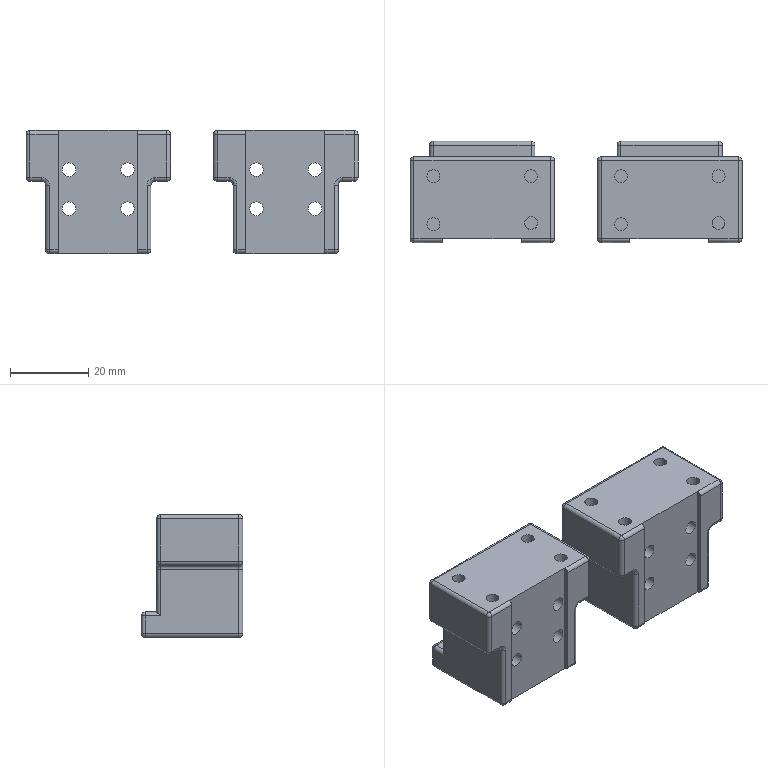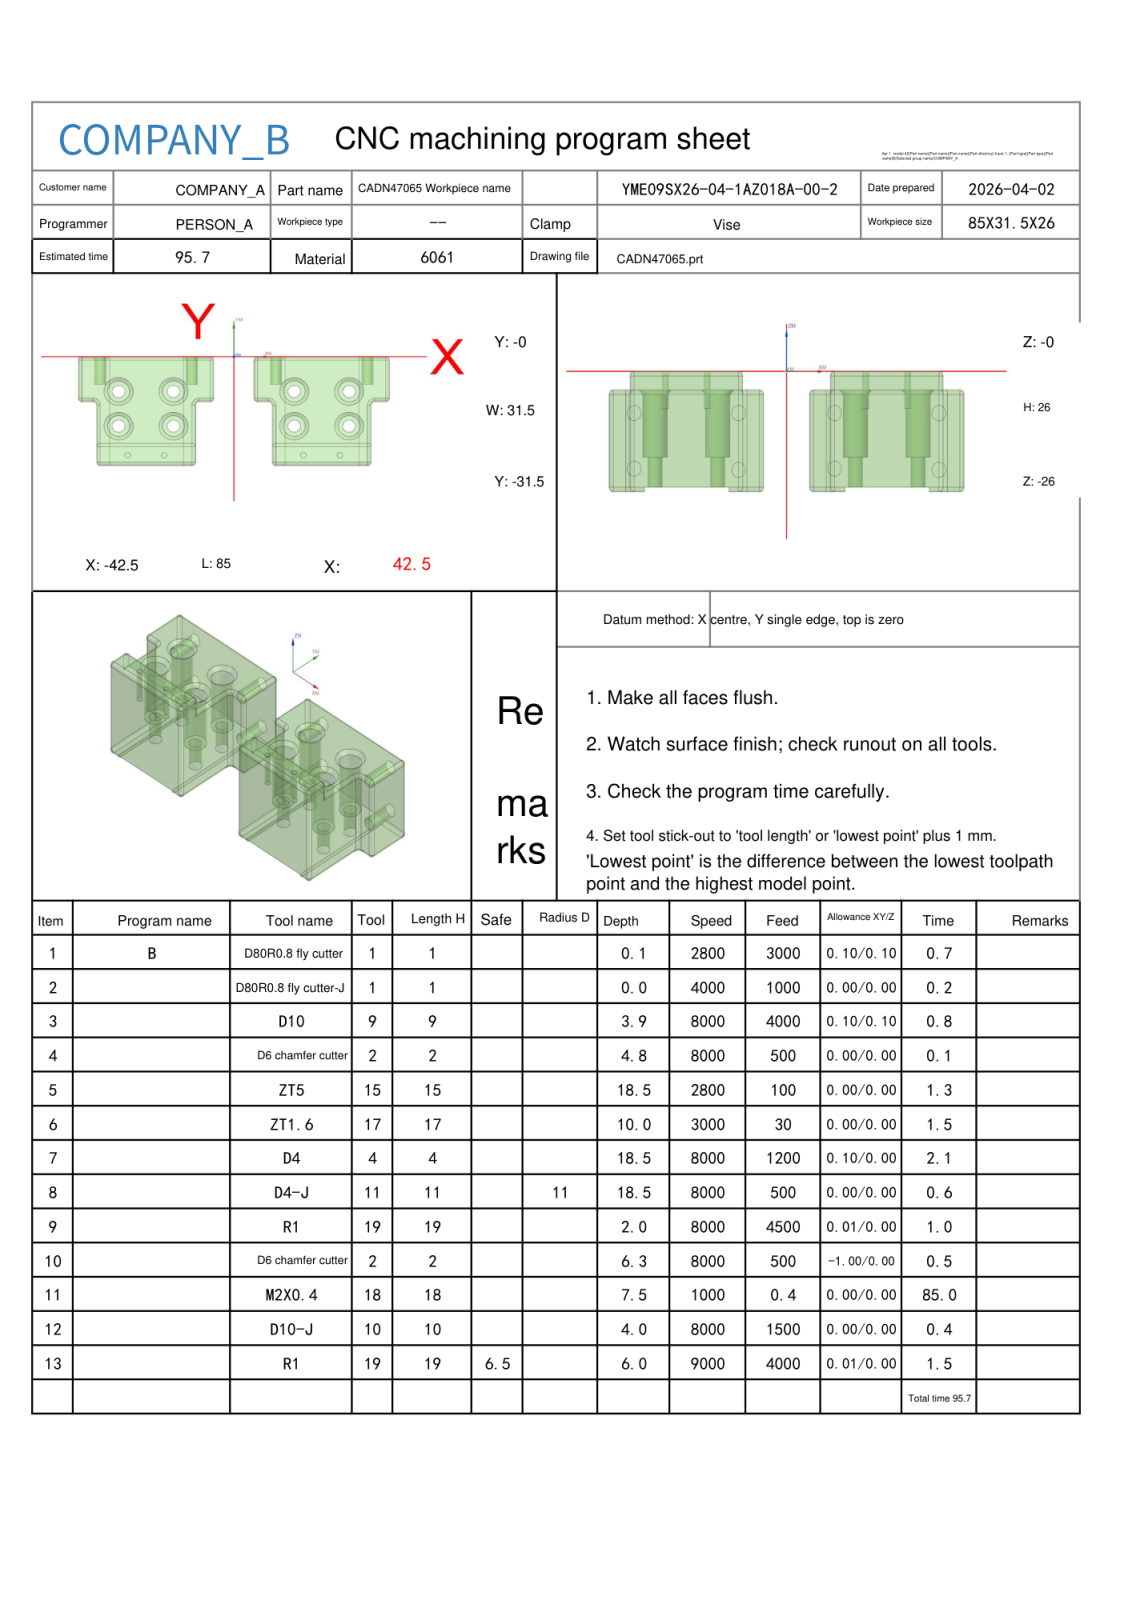NC program | NX | posted by the shop | part box 85 x 26 x 31.5 mm
Lines 1 to 1233 of 12542:
%
O0001
(Machine time: 173.10 MIN)
(===Total Tool:10===)
(T1=D80R0.8 fly cutter D=80.  R=0.8  D-  H01 Z=-0.   )
(T9=D10     D=10.  R=0.   D-  H09 Z=-3.9  )
(T2=D6 chamfer cutter   D=6.   R=0.   D-  H02 Z=-6.3  )
(T15=ZT5    D=5.   DR_a=118 D-  H15 Z=-18.51)
(T17=ZT1.6  D=1.6  DR_a=118 D-  H17 Z=-10.  )
(T4=D4      D=4.   R=0.   D-  H04 Z=-18.51)
(T11=D4-J   D=4.   R=0.   D11 H11 Z=-18.51)
(T19=R1     D=2.   R=1.   D-  H19 Z=-6.   )
(T18=M2X0.4 D=1.6  DR_a=180 D-  H18 Z=-7.5  )
(T10=D10-J  D=10.  R=0.   D10 H10 Z=-4.   )
G80 G90 G17 G49 G40
G91 G28 Z0
M01
N1 T01 M06
(D80R0.8 fly cutter  D=80. R=0.8 H=01 ce=0.10 di=0.10)
G00 G90 G54 X94.57 Y-13.688 M03 S2800
G43 H01 Z20.
M08
Z5.337
G01 Z3.337 F3000.
X82.551 Y-13.943
X-82.235 Y-17.444
X-94.29 Y-17.7
Z5.337
G00 X94.57 Y-13.688
Z4.875
G01 Z2.875
X82.551 Y-13.943
X-82.235 Y-17.444
X-94.29 Y-17.7
Z4.875
G00 X94.57 Y-13.688
Z4.412
G01 Z2.412
X82.551 Y-13.943
X-82.235 Y-17.444
X-94.29 Y-17.7
Z4.412
G00 X94.57 Y-13.688
Z3.95
G01 Z1.95
X82.551 Y-13.943
X-82.235 Y-17.444
X-94.29 Y-17.7
Z3.95
G00 Z20.
X94.57 Y-13.688
Z3.487
G01 Z1.487
X82.551 Y-13.943
X-82.235 Y-17.444
X-94.29 Y-17.7
Z3.487
G00 Z20.
X94.57 Y-13.688
Z3.025
G01 Z1.025
X82.551 Y-13.943
X-82.235 Y-17.444
X-94.29 Y-17.7
Z3.025
G00 Z20.
X94.57 Y-13.688
Z2.562
G01 Z.562
X82.551 Y-13.943
X-82.235 Y-17.444
X-94.29 Y-17.7
Z2.562
G00 Z20.
X94.57 Y-13.688
Z2.1
G01 Z.1
X82.551 Y-13.943
X-82.235 Y-17.444
X-94.29 Y-17.7
Z2.1
G00 Z20.
G91 G28 Z0.0
M05
M09
G91 G28 Z0.0
M01
N2 T01 M06
(D80R0.8 fly cutter-J  D=80. R=0.8 H=01 ce=0.00 di=0.00)
G00 G90 G54 X94.472 Y-13.691 M03 S4000
G43 H01 Z20.
M08
Z2.
G01 Z0.0 F1000.
X82.453 Y-13.947
X-82.136 Y-17.441
X-94.192 Y-17.696
Z2.
G00 Z20.
G91 G28 Z0.0
M05
M09
G91 G28 Z0.0
M01
N3 T09 M06
(D10  D=10. R=0. H=09 ce=0.10 di=0.10)
G00 G90 G54 X0.0 Y7. M03 S8000
G43 H09 Z13.8
M08
Z.943
G01 Z-.557 F4000.
Y3.9
X46.4
Y-16.9
X41.4
Y-20.659
Y-22.322
G03 X36.5 Y-19.855 I-4.9 J-3.633
G01 X11.5
G03 X6.6 Y-22.322 I0.0 J-6.1
G01 Y-16.9
X-6.6
Y-20.658
Y-22.322
G03 X-11.5 Y-19.855 I-4.9 J-3.633
G01 X-36.5
G03 X-41.4 Y-22.322 I0.0 J-6.1
G01 Y-20.659
Y-16.9
X-46.4
Y3.9
X-3.035
G02 X-2.203 Y3.455 I-.001 J-1.
G01 X2.203 Y-3.155
G03 X3.035 Y-3.6 I.832 J.555
G01 X37.903
G02 X38.9 Y-4.597 I-.003 J-1.
G01 Y-9.157
G02 X38.314 Y-10.064 I-1. J.003
G03 X35.714 Y-12.009 I3.086 J-6.836
G02 X34.96 Y-12.355 I-.756 J.654
G01 X13.04
G02 X12.286 Y-12.009 I.003 J1.
G03 X6.6 Y-9.4 I-5.686 J-4.891
G01 X-6.6
G03 X-12.286 Y-12.009 I0.0 J-7.5
G02 X-13.04 Y-12.355 I-.756 J.654
G01 X-34.96
G02 X-35.714 Y-12.009 I.003 J1.
G03 X-38.314 Y-10.064 I-5.686 J-4.891
G02 X-38.9 Y-9.157 I.414 J.91
G01 Y-4.597
G02 X-37.903 Y-3.6 I1. J-.003
G01 X0.0
X.5
Y7.
Z.943
G00 X0.0
Z.386
G01 Z-1.114
Y3.9
X46.4
Y-16.9
X41.4
Y-20.659
Y-22.322
G03 X36.5 Y-19.855 I-4.9 J-3.633
G01 X11.5
G03 X6.6 Y-22.322 I0.0 J-6.1
G01 Y-16.9
X-6.6
Y-20.658
Y-22.322
G03 X-11.5 Y-19.855 I-4.9 J-3.633
G01 X-36.5
G03 X-41.4 Y-22.322 I0.0 J-6.1
G01 Y-20.659
Y-16.9
X-46.4
Y3.9
X-3.035
G02 X-2.203 Y3.455 I-.001 J-1.
G01 X2.203 Y-3.155
G03 X3.035 Y-3.6 I.832 J.555
G01 X37.903
G02 X38.9 Y-4.597 I-.003 J-1.
G01 Y-9.157
G02 X38.314 Y-10.064 I-1. J.003
G03 X35.714 Y-12.009 I3.086 J-6.836
G02 X34.96 Y-12.355 I-.756 J.654
G01 X13.04
G02 X12.286 Y-12.009 I.003 J1.
G03 X6.6 Y-9.4 I-5.686 J-4.891
G01 X-6.6
G03 X-12.286 Y-12.009 I0.0 J-7.5
G02 X-13.04 Y-12.355 I-.756 J.654
G01 X-34.96
G02 X-35.714 Y-12.009 I.003 J1.
G03 X-38.314 Y-10.064 I-5.686 J-4.891
G02 X-38.9 Y-9.157 I.414 J.91
G01 Y-4.597
G02 X-37.903 Y-3.6 I1. J-.003
G01 X0.0
X.5
Y7.
Z.386
G00 X0.0
Z-.171
G01 Z-1.671
Y3.9
X46.4
Y-16.9
X41.4
Y-20.659
Y-22.322
G03 X36.5 Y-19.855 I-4.9 J-3.633
G01 X11.5
G03 X6.6 Y-22.322 I0.0 J-6.1
G01 Y-16.9
X-6.6
Y-20.658
Y-22.322
G03 X-11.5 Y-19.855 I-4.9 J-3.633
G01 X-36.5
G03 X-41.4 Y-22.322 I0.0 J-6.1
G01 Y-20.659
Y-16.9
X-46.4
Y3.9
X-3.035
G02 X-2.203 Y3.455 I-.001 J-1.
G01 X2.203 Y-3.155
G03 X3.035 Y-3.6 I.832 J.555
G01 X37.903
G02 X38.9 Y-4.597 I-.003 J-1.
G01 Y-9.157
G02 X38.314 Y-10.064 I-1. J.003
G03 X35.714 Y-12.009 I3.086 J-6.836
G02 X34.96 Y-12.355 I-.756 J.654
G01 X13.04
G02 X12.286 Y-12.009 I.003 J1.
G03 X6.6 Y-9.4 I-5.686 J-4.891
G01 X-6.6
G03 X-12.286 Y-12.009 I0.0 J-7.5
G02 X-13.04 Y-12.355 I-.756 J.654
G01 X-34.96
G02 X-35.714 Y-12.009 I.003 J1.
G03 X-38.314 Y-10.064 I-5.686 J-4.891
G02 X-38.9 Y-9.157 I.414 J.91
G01 Y-4.597
G02 X-37.903 Y-3.6 I1. J-.003
G01 X0.0
X.5
Y7.
Z-.171
G00 X0.0
Z-.729
G01 Z-2.229
Y3.9
X46.4
Y-16.9
X41.4
Y-20.659
Y-22.322
G03 X36.5 Y-19.855 I-4.9 J-3.633
G01 X11.5
G03 X6.6 Y-22.322 I0.0 J-6.1
G01 Y-16.9
X-6.6
Y-20.658
Y-22.322
G03 X-11.5 Y-19.855 I-4.9 J-3.633
G01 X-36.5
G03 X-41.4 Y-22.322 I0.0 J-6.1
G01 Y-20.659
Y-16.9
X-46.4
Y3.9
X-3.035
G02 X-2.203 Y3.455 I-.001 J-1.
G01 X2.203 Y-3.155
G03 X3.035 Y-3.6 I.832 J.555
G01 X37.903
G02 X38.9 Y-4.597 I-.003 J-1.
G01 Y-9.157
G02 X38.314 Y-10.064 I-1. J.003
G03 X35.714 Y-12.009 I3.086 J-6.836
G02 X34.96 Y-12.355 I-.756 J.654
G01 X13.04
G02 X12.286 Y-12.009 I.003 J1.
G03 X6.6 Y-9.4 I-5.686 J-4.891
G01 X-6.6
G03 X-12.286 Y-12.009 I0.0 J-7.5
G02 X-13.04 Y-12.355 I-.756 J.654
G01 X-34.96
G02 X-35.714 Y-12.009 I.003 J1.
G03 X-38.314 Y-10.064 I-5.686 J-4.891
G02 X-38.9 Y-9.157 I.414 J.91
G01 Y-4.597
G02 X-37.903 Y-3.6 I1. J-.003
G01 X0.0
X.5
Y7.
Z-.729
G00 X0.0
Z-1.286
G01 Z-2.786
Y3.9
X46.4
Y-16.9
X41.4
Y-20.659
Y-22.322
G03 X36.5 Y-19.855 I-4.9 J-3.633
G01 X11.5
G03 X6.6 Y-22.322 I0.0 J-6.1
G01 Y-16.9
X-6.6
Y-20.658
Y-22.322
G03 X-11.5 Y-19.855 I-4.9 J-3.633
G01 X-36.5
G03 X-41.4 Y-22.322 I0.0 J-6.1
G01 Y-20.659
Y-16.9
X-46.4
Y3.9
X-3.035
G02 X-2.203 Y3.455 I-.001 J-1.
G01 X2.203 Y-3.155
G03 X3.035 Y-3.6 I.832 J.555
G01 X37.903
G02 X38.9 Y-4.597 I-.003 J-1.
G01 Y-9.157
G02 X38.314 Y-10.064 I-1. J.003
G03 X35.714 Y-12.009 I3.086 J-6.836
G02 X34.96 Y-12.355 I-.756 J.654
G01 X13.04
G02 X12.286 Y-12.009 I.003 J1.
G03 X6.6 Y-9.4 I-5.686 J-4.891
G01 X-6.6
G03 X-12.286 Y-12.009 I0.0 J-7.5
G02 X-13.04 Y-12.355 I-.756 J.654
G01 X-34.96
G02 X-35.714 Y-12.009 I.003 J1.
G03 X-38.314 Y-10.064 I-5.686 J-4.891
G02 X-38.9 Y-9.157 I.414 J.91
G01 Y-4.597
G02 X-37.903 Y-3.6 I1. J-.003
G01 X0.0
X.5
Y7.
Z-1.286
G00 X0.0
Z-1.843
G01 Z-3.343
Y3.9
X46.4
Y-16.9
X41.4
Y-20.659
Y-22.322
G03 X36.5 Y-19.855 I-4.9 J-3.633
G01 X11.5
G03 X6.6 Y-22.322 I0.0 J-6.1
G01 Y-16.9
X-6.6
Y-20.658
Y-22.322
G03 X-11.5 Y-19.855 I-4.9 J-3.633
G01 X-36.5
G03 X-41.4 Y-22.322 I0.0 J-6.1
G01 Y-20.659
Y-16.9
X-46.4
Y3.9
X-3.035
G02 X-2.203 Y3.455 I-.001 J-1.
G01 X2.203 Y-3.155
G03 X3.035 Y-3.6 I.832 J.555
G01 X37.903
G02 X38.9 Y-4.597 I-.003 J-1.
G01 Y-9.157
G02 X38.314 Y-10.064 I-1. J.003
G03 X35.714 Y-12.009 I3.086 J-6.836
G02 X34.96 Y-12.355 I-.756 J.654
G01 X13.04
G02 X12.286 Y-12.009 I.003 J1.
G03 X6.6 Y-9.4 I-5.686 J-4.891
G01 X-6.6
G03 X-12.286 Y-12.009 I0.0 J-7.5
G02 X-13.04 Y-12.355 I-.756 J.654
G01 X-34.96
G02 X-35.714 Y-12.009 I.003 J1.
G03 X-38.314 Y-10.064 I-5.686 J-4.891
G02 X-38.9 Y-9.157 I.414 J.91
G01 Y-4.597
G02 X-37.903 Y-3.6 I1. J-.003
G01 X0.0
X.5
Y7.
Z-1.843
G00 X0.0
Z-2.4
G01 Z-3.9
Y3.9
X46.4
Y-16.9
X41.4
Y-20.659
Y-22.322
G03 X36.5 Y-19.855 I-4.9 J-3.633
G01 X11.5
G03 X6.6 Y-22.322 I0.0 J-6.1
G01 Y-16.9
X-6.6
Y-20.658
Y-22.322
G03 X-11.5 Y-19.855 I-4.9 J-3.633
G01 X-36.5
G03 X-41.4 Y-22.322 I0.0 J-6.1
G01 Y-20.659
Y-16.9
X-46.4
Y3.9
X-3.035
G02 X-2.203 Y3.455 I-.001 J-1.
G01 X2.203 Y-3.155
G03 X3.035 Y-3.6 I.832 J.555
G01 X37.903
G02 X38.9 Y-4.597 I-.003 J-1.
G01 Y-9.157
G02 X38.314 Y-10.064 I-1. J.003
G03 X35.714 Y-12.009 I3.086 J-6.836
G02 X34.96 Y-12.355 I-.756 J.654
G01 X13.04
G02 X12.286 Y-12.009 I.003 J1.
G03 X6.6 Y-9.4 I-5.686 J-4.891
G01 X-6.6
G03 X-12.286 Y-12.009 I0.0 J-7.5
G02 X-13.04 Y-12.355 I-.756 J.654
G01 X-34.96
G02 X-35.714 Y-12.009 I.003 J1.
G03 X-38.314 Y-10.064 I-5.686 J-4.891
G02 X-38.9 Y-9.157 I.414 J.91
G01 Y-4.597
G02 X-37.903 Y-3.6 I1. J-.003
G01 X0.0
X.5
Y7.
Z-2.4
G00 Z13.8
G91 G28 Z0.0
M05
M09
G91 G28 Z0.0
M01
N4 T02 M06
(D6 chamfer cutter  D=6. R=0. H=02 ce=0.00 di=0.10)
G00 G90 G54 X-31.502 Y-10.05 M03 S8000
G43 H02 Z20.
M08
G98 G81 X-31.502 Y-10.05 Z-4.8 R-3. F500.
Y-20.05
X-29.011 Y-28.455 Z-.8 R1.
X-19.011
X-16.502 Y-20.05 Z-4.8 R-3.
Y-10.05
X16.498
Y-20.05
X18.989 Y-28.455 Z-.8 R1.
X28.989
X31.498 Y-20.05 Z-4.8 R-3.
Y-10.05
G80
G00 Z20.
G91 G28 Z0.0
M05
M09
G91 G28 Z0.0
M01
N5 T15 M06
(ZT5 D=5. DR_a=118 H=15)
G00 G90 G54 X-31.502 Y-20.05 M03 S2800
G43 H15 Z20.
M08
G98 G83 X-31.502 Y-20.05 Z-18.51 R-3. F100. Q2.
Y-10.05
X-16.502
Y-20.05
X16.498
Y-10.05
X31.498
Y-20.05
G80
G00 Z20.
G91 G28 Z0.0
M05
M09
G91 G28 Z0.0
M01
N6 T17 M06
(ZT1.6 D=1.6 DR_a=118 H=17)
G00 G90 G54 X-29.011 Y-28.455 M03 S3000
G43 H17 Z20.
M08
G98 G83 X-29.011 Y-28.455 Z-10. R1. F30. Q1.
X-19.011
X18.989
X28.989
G80
G00 Z20.
G91 G28 Z0.0
M05
M09
G91 G28 Z0.0
M01
N7 T04 M06
(D4  D=4. R=0. H=04 ce=0.10 di=0.00)
G00 G90 G54 X-16.502 Y-10.05 M03 S8000
G43 H04 Z20.
M08
Z-2.5
G03 X-16.952 Y-9.6 I-.45 J0.0 F1200.
X-17.402 Y-10.05 I0.0 J-.45
X-17.402 Y-10.05 Z-2.8 I.9 J0.0
X-17.402 Y-10.05 Z-3.1 I.9 J0.0
X-17.402 Y-10.05 Z-3.4 I.9 J0.0
X-17.402 Y-10.05 Z-3.7 I.9 J0.0
X-17.402 Y-10.05 Z-4. I.9 J0.0
X-17.402 Y-10.05 Z-4.3 I.9 J0.0
X-17.402 Y-10.05 Z-4.6 I.9 J0.0
X-17.402 Y-10.05 Z-4.9 I.9 J0.0
X-17.402 Y-10.05 Z-5.2 I.9 J0.0
X-17.402 Y-10.05 Z-5.5 I.9 J0.0
X-17.402 Y-10.05 Z-5.8 I.9 J0.0
X-17.402 Y-10.05 Z-6.1 I.9 J0.0
X-17.402 Y-10.05 Z-6.4 I.9 J0.0
X-17.402 Y-10.05 Z-6.7 I.9 J0.0
X-17.402 Y-10.05 Z-7. I.9 J0.0
X-17.402 Y-10.05 Z-7.3 I.9 J0.0
X-17.402 Y-10.05 Z-7.6 I.9 J0.0
X-17.402 Y-10.05 Z-7.9 I.9 J0.0
X-17.402 Y-10.05 Z-8.2 I.9 J0.0
X-17.402 Y-10.05 Z-8.5 I.9 J0.0
X-17.402 Y-10.05 Z-8.8 I.9 J0.0
X-17.402 Y-10.05 Z-9.1 I.9 J0.0
X-17.402 Y-10.05 Z-9.4 I.9 J0.0
X-17.402 Y-10.05 Z-9.7 I.9 J0.0
X-17.402 Y-10.05 Z-10. I.9 J0.0
X-17.402 Y-10.05 Z-10.3 I.9 J0.0
X-17.402 Y-10.05 Z-10.6 I.9 J0.0
X-17.402 Y-10.05 Z-10.9 I.9 J0.0
X-17.402 Y-10.05 Z-11.2 I.9 J0.0
X-17.402 Y-10.05 Z-11.5 I.9 J0.0
X-17.402 Y-10.05 Z-11.8 I.9 J0.0
X-17.402 Y-10.05 Z-12.1 I.9 J0.0
X-17.402 Y-10.05 Z-12.4 I.9 J0.0
X-17.402 Y-10.05 Z-12.7 I.9 J0.0
X-17.402 Y-10.05 Z-13. I.9 J0.0
X-17.402 Y-10.05 Z-13.3 I.9 J0.0
X-17.402 Y-10.05 Z-13.6 I.9 J0.0
X-17.402 Y-10.05 Z-13.9 I.9 J0.0
X-17.402 Y-10.05 Z-14.2 I.9 J0.0
X-17.402 Y-10.05 Z-14.5 I.9 J0.0
X-17.402 Y-10.05 Z-14.8 I.9 J0.0
X-17.402 Y-10.05 Z-15.1 I.9 J0.0
X-17.402 Y-10.05 Z-15.4 I.9 J0.0
X-17.402 Y-10.05 Z-15.7 I.9 J0.0
X-17.402 Y-10.05 Z-16. I.9 J0.0
X-17.402 Y-10.05 Z-16.3 I.9 J0.0
X-17.402 Y-10.05 Z-16.6 I.9 J0.0
X-17.402 Y-10.05 Z-16.9 I.9 J0.0
X-17.402 Y-10.05 Z-17.2 I.9 J0.0
X-17.402 Y-10.05 Z-17.5 I.9 J0.0
X-17.402 Y-10.05 Z-17.8 I.9 J0.0
X-17.402 Y-10.05 Z-18.1 I.9 J0.0
X-17.402 Y-10.05 Z-18.4 I.9 J0.0
X-15.901 Y-10.719 Z-18.51 I.9 J0.0
X-15.602 Y-10.05 I-.602 J.669
X-16.502 Y-9.15 I-.9 J0.0
X-17.402 Y-10.05 I0.0 J-.9
X-16.502 Y-10.95 I.9 J0.0
X-15.901 Y-10.719 I0.0 J.9
X-15.752 Y-10.385 I-.301 J.335
X-16.202 Y-9.935 I-.45 J0.0
X-16.502 Y-10.05 I0.0 J-.45
G00 Z20.
X-31.502
Z-2.5
G03 X-31.952 Y-9.6 I-.45 J0.0
X-32.402 Y-10.05 I0.0 J-.45
X-32.402 Y-10.05 Z-2.8 I.9 J0.0
X-32.402 Y-10.05 Z-3.1 I.9 J0.0
X-32.402 Y-10.05 Z-3.4 I.9 J0.0
X-32.402 Y-10.05 Z-3.7 I.9 J0.0
X-32.402 Y-10.05 Z-4. I.9 J0.0
X-32.402 Y-10.05 Z-4.3 I.9 J0.0
X-32.402 Y-10.05 Z-4.6 I.9 J0.0
X-32.402 Y-10.05 Z-4.9 I.9 J0.0
X-32.402 Y-10.05 Z-5.2 I.9 J0.0
X-32.402 Y-10.05 Z-5.5 I.9 J0.0
X-32.402 Y-10.05 Z-5.8 I.9 J0.0
X-32.402 Y-10.05 Z-6.1 I.9 J0.0
X-32.402 Y-10.05 Z-6.4 I.9 J0.0
X-32.402 Y-10.05 Z-6.7 I.9 J0.0
X-32.402 Y-10.05 Z-7. I.9 J0.0
X-32.402 Y-10.05 Z-7.3 I.9 J0.0
X-32.402 Y-10.05 Z-7.6 I.9 J0.0
X-32.402 Y-10.05 Z-7.9 I.9 J0.0
X-32.402 Y-10.05 Z-8.2 I.9 J0.0
X-32.402 Y-10.05 Z-8.5 I.9 J0.0
X-32.402 Y-10.05 Z-8.8 I.9 J0.0
X-32.402 Y-10.05 Z-9.1 I.9 J0.0
X-32.402 Y-10.05 Z-9.4 I.9 J0.0
X-32.402 Y-10.05 Z-9.7 I.9 J0.0
X-32.402 Y-10.05 Z-10. I.9 J0.0
X-32.402 Y-10.05 Z-10.3 I.9 J0.0
X-32.402 Y-10.05 Z-10.6 I.9 J0.0
X-32.402 Y-10.05 Z-10.9 I.9 J0.0
X-32.402 Y-10.05 Z-11.2 I.9 J0.0
X-32.402 Y-10.05 Z-11.5 I.9 J0.0
X-32.402 Y-10.05 Z-11.8 I.9 J0.0
X-32.402 Y-10.05 Z-12.1 I.9 J0.0
X-32.402 Y-10.05 Z-12.4 I.9 J0.0
X-32.402 Y-10.05 Z-12.7 I.9 J0.0
X-32.402 Y-10.05 Z-13. I.9 J0.0
X-32.402 Y-10.05 Z-13.3 I.9 J0.0
X-32.402 Y-10.05 Z-13.6 I.9 J0.0
X-32.402 Y-10.05 Z-13.9 I.9 J0.0
X-32.402 Y-10.05 Z-14.2 I.9 J0.0
X-32.402 Y-10.05 Z-14.5 I.9 J0.0
X-32.402 Y-10.05 Z-14.8 I.9 J0.0
X-32.402 Y-10.05 Z-15.1 I.9 J0.0
X-32.402 Y-10.05 Z-15.4 I.9 J0.0
X-32.402 Y-10.05 Z-15.7 I.9 J0.0
X-32.402 Y-10.05 Z-16. I.9 J0.0
X-32.402 Y-10.05 Z-16.3 I.9 J0.0
X-32.402 Y-10.05 Z-16.6 I.9 J0.0
X-32.402 Y-10.05 Z-16.9 I.9 J0.0
X-32.402 Y-10.05 Z-17.2 I.9 J0.0
X-32.402 Y-10.05 Z-17.5 I.9 J0.0
X-32.402 Y-10.05 Z-17.8 I.9 J0.0
X-32.402 Y-10.05 Z-18.1 I.9 J0.0
X-32.402 Y-10.05 Z-18.4 I.9 J0.0
X-30.901 Y-10.719 Z-18.51 I.9 J0.0
X-30.602 Y-10.05 I-.602 J.669
X-31.502 Y-9.15 I-.9 J0.0
X-32.402 Y-10.05 I0.0 J-.9
X-31.502 Y-10.95 I.9 J0.0
X-30.901 Y-10.719 I0.0 J.9
X-30.752 Y-10.385 I-.301 J.335
X-31.202 Y-9.935 I-.45 J0.0
X-31.502 Y-10.05 I0.0 J-.45
G00 Z20.
Y-20.05
Z-2.5
G03 X-31.952 Y-19.6 I-.45 J0.0
X-32.402 Y-20.05 I0.0 J-.45
X-32.402 Y-20.05 Z-2.8 I.9 J0.0
X-32.402 Y-20.05 Z-3.1 I.9 J0.0
X-32.402 Y-20.05 Z-3.4 I.9 J0.0
X-32.402 Y-20.05 Z-3.7 I.9 J0.0
X-32.402 Y-20.05 Z-4. I.9 J0.0
X-32.402 Y-20.05 Z-4.3 I.9 J0.0
X-32.402 Y-20.05 Z-4.6 I.9 J0.0
X-32.402 Y-20.05 Z-4.9 I.9 J0.0
X-32.402 Y-20.05 Z-5.2 I.9 J0.0
X-32.402 Y-20.05 Z-5.5 I.9 J0.0
X-32.402 Y-20.05 Z-5.8 I.9 J0.0
X-32.402 Y-20.05 Z-6.1 I.9 J0.0
X-32.402 Y-20.05 Z-6.4 I.9 J0.0
X-32.402 Y-20.05 Z-6.7 I.9 J0.0
X-32.402 Y-20.05 Z-7. I.9 J0.0
X-32.402 Y-20.05 Z-7.3 I.9 J0.0
X-32.402 Y-20.05 Z-7.6 I.9 J0.0
X-32.402 Y-20.05 Z-7.9 I.9 J0.0
X-32.402 Y-20.05 Z-8.2 I.9 J0.0
X-32.402 Y-20.05 Z-8.5 I.9 J0.0
X-32.402 Y-20.05 Z-8.8 I.9 J0.0
X-32.402 Y-20.05 Z-9.1 I.9 J0.0
X-32.402 Y-20.05 Z-9.4 I.9 J0.0
X-32.402 Y-20.05 Z-9.7 I.9 J0.0
X-32.402 Y-20.05 Z-10. I.9 J0.0
X-32.402 Y-20.05 Z-10.3 I.9 J0.0
X-32.402 Y-20.05 Z-10.6 I.9 J0.0
X-32.402 Y-20.05 Z-10.9 I.9 J0.0
X-32.402 Y-20.05 Z-11.2 I.9 J0.0
X-32.402 Y-20.05 Z-11.5 I.9 J0.0
X-32.402 Y-20.05 Z-11.8 I.9 J0.0
X-32.402 Y-20.05 Z-12.1 I.9 J0.0
X-32.402 Y-20.05 Z-12.4 I.9 J0.0
X-32.402 Y-20.05 Z-12.7 I.9 J0.0
X-32.402 Y-20.05 Z-13. I.9 J0.0
X-32.402 Y-20.05 Z-13.3 I.9 J0.0
X-32.402 Y-20.05 Z-13.6 I.9 J0.0
X-32.402 Y-20.05 Z-13.9 I.9 J0.0
X-32.402 Y-20.05 Z-14.2 I.9 J0.0
X-32.402 Y-20.05 Z-14.5 I.9 J0.0
X-32.402 Y-20.05 Z-14.8 I.9 J0.0
X-32.402 Y-20.05 Z-15.1 I.9 J0.0
X-32.402 Y-20.05 Z-15.4 I.9 J0.0
X-32.402 Y-20.05 Z-15.7 I.9 J0.0
X-32.402 Y-20.05 Z-16. I.9 J0.0
X-32.402 Y-20.05 Z-16.3 I.9 J0.0
X-32.402 Y-20.05 Z-16.6 I.9 J0.0
X-32.402 Y-20.05 Z-16.9 I.9 J0.0
X-32.402 Y-20.05 Z-17.2 I.9 J0.0
X-32.402 Y-20.05 Z-17.5 I.9 J0.0
X-32.402 Y-20.05 Z-17.8 I.9 J0.0
X-32.402 Y-20.05 Z-18.1 I.9 J0.0
X-32.402 Y-20.05 Z-18.4 I.9 J0.0
X-30.901 Y-20.719 Z-18.51 I.9 J0.0
X-30.602 Y-20.05 I-.602 J.669
X-31.502 Y-19.15 I-.9 J0.0
X-32.402 Y-20.05 I0.0 J-.9
X-31.502 Y-20.95 I.9 J0.0
X-30.901 Y-20.719 I0.0 J.9
X-30.752 Y-20.385 I-.301 J.335
X-31.202 Y-19.935 I-.45 J0.0
X-31.502 Y-20.05 I0.0 J-.45
G00 Z20.
X-16.502
Z-2.5
G03 X-16.952 Y-19.6 I-.45 J0.0
X-17.402 Y-20.05 I0.0 J-.45
X-17.402 Y-20.05 Z-2.8 I.9 J0.0
X-17.402 Y-20.05 Z-3.1 I.9 J0.0
X-17.402 Y-20.05 Z-3.4 I.9 J0.0
X-17.402 Y-20.05 Z-3.7 I.9 J0.0
X-17.402 Y-20.05 Z-4. I.9 J0.0
X-17.402 Y-20.05 Z-4.3 I.9 J0.0
X-17.402 Y-20.05 Z-4.6 I.9 J0.0
X-17.402 Y-20.05 Z-4.9 I.9 J0.0
X-17.402 Y-20.05 Z-5.2 I.9 J0.0
X-17.402 Y-20.05 Z-5.5 I.9 J0.0
X-17.402 Y-20.05 Z-5.8 I.9 J0.0
X-17.402 Y-20.05 Z-6.1 I.9 J0.0
X-17.402 Y-20.05 Z-6.4 I.9 J0.0
X-17.402 Y-20.05 Z-6.7 I.9 J0.0
X-17.402 Y-20.05 Z-7. I.9 J0.0
X-17.402 Y-20.05 Z-7.3 I.9 J0.0
X-17.402 Y-20.05 Z-7.6 I.9 J0.0
X-17.402 Y-20.05 Z-7.9 I.9 J0.0
X-17.402 Y-20.05 Z-8.2 I.9 J0.0
X-17.402 Y-20.05 Z-8.5 I.9 J0.0
X-17.402 Y-20.05 Z-8.8 I.9 J0.0
X-17.402 Y-20.05 Z-9.1 I.9 J0.0
X-17.402 Y-20.05 Z-9.4 I.9 J0.0
X-17.402 Y-20.05 Z-9.7 I.9 J0.0
X-17.402 Y-20.05 Z-10. I.9 J0.0
X-17.402 Y-20.05 Z-10.3 I.9 J0.0
X-17.402 Y-20.05 Z-10.6 I.9 J0.0
X-17.402 Y-20.05 Z-10.9 I.9 J0.0
X-17.402 Y-20.05 Z-11.2 I.9 J0.0
X-17.402 Y-20.05 Z-11.5 I.9 J0.0
X-17.402 Y-20.05 Z-11.8 I.9 J0.0
X-17.402 Y-20.05 Z-12.1 I.9 J0.0
X-17.402 Y-20.05 Z-12.4 I.9 J0.0
X-17.402 Y-20.05 Z-12.7 I.9 J0.0
X-17.402 Y-20.05 Z-13. I.9 J0.0
X-17.402 Y-20.05 Z-13.3 I.9 J0.0
X-17.402 Y-20.05 Z-13.6 I.9 J0.0
X-17.402 Y-20.05 Z-13.9 I.9 J0.0
X-17.402 Y-20.05 Z-14.2 I.9 J0.0
X-17.402 Y-20.05 Z-14.5 I.9 J0.0
X-17.402 Y-20.05 Z-14.8 I.9 J0.0
X-17.402 Y-20.05 Z-15.1 I.9 J0.0
X-17.402 Y-20.05 Z-15.4 I.9 J0.0
X-17.402 Y-20.05 Z-15.7 I.9 J0.0
X-17.402 Y-20.05 Z-16. I.9 J0.0
X-17.402 Y-20.05 Z-16.3 I.9 J0.0
X-17.402 Y-20.05 Z-16.6 I.9 J0.0
X-17.402 Y-20.05 Z-16.9 I.9 J0.0
X-17.402 Y-20.05 Z-17.2 I.9 J0.0
X-17.402 Y-20.05 Z-17.5 I.9 J0.0
X-17.402 Y-20.05 Z-17.8 I.9 J0.0
X-17.402 Y-20.05 Z-18.1 I.9 J0.0
X-17.402 Y-20.05 Z-18.4 I.9 J0.0
X-15.901 Y-20.719 Z-18.51 I.9 J0.0
X-15.602 Y-20.05 I-.602 J.669
X-16.502 Y-19.15 I-.9 J0.0
X-17.402 Y-20.05 I0.0 J-.9
X-16.502 Y-20.95 I.9 J0.0
X-15.901 Y-20.719 I0.0 J.9
X-15.752 Y-20.385 I-.301 J.335
X-16.202 Y-19.935 I-.45 J0.0
X-16.502 Y-20.05 I0.0 J-.45
G00 Z20.
X16.498
Z-2.5
G03 X16.048 Y-19.6 I-.45 J0.0
X15.598 Y-20.05 I0.0 J-.45
X15.598 Y-20.05 Z-2.8 I.9 J0.0
X15.598 Y-20.05 Z-3.1 I.9 J0.0
X15.598 Y-20.05 Z-3.4 I.9 J0.0
X15.598 Y-20.05 Z-3.7 I.9 J0.0
X15.598 Y-20.05 Z-4. I.9 J0.0
X15.598 Y-20.05 Z-4.3 I.9 J0.0
X15.598 Y-20.05 Z-4.6 I.9 J0.0
X15.598 Y-20.05 Z-4.9 I.9 J0.0
X15.598 Y-20.05 Z-5.2 I.9 J0.0
X15.598 Y-20.05 Z-5.5 I.9 J0.0
X15.598 Y-20.05 Z-5.8 I.9 J0.0
X15.598 Y-20.05 Z-6.1 I.9 J0.0
X15.598 Y-20.05 Z-6.4 I.9 J0.0
X15.598 Y-20.05 Z-6.7 I.9 J0.0
X15.598 Y-20.05 Z-7. I.9 J0.0
X15.598 Y-20.05 Z-7.3 I.9 J0.0
X15.598 Y-20.05 Z-7.6 I.9 J0.0
X15.598 Y-20.05 Z-7.9 I.9 J0.0
X15.598 Y-20.05 Z-8.2 I.9 J0.0
X15.598 Y-20.05 Z-8.5 I.9 J0.0
X15.598 Y-20.05 Z-8.8 I.9 J0.0
X15.598 Y-20.05 Z-9.1 I.9 J0.0
X15.598 Y-20.05 Z-9.4 I.9 J0.0
X15.598 Y-20.05 Z-9.7 I.9 J0.0
X15.598 Y-20.05 Z-10. I.9 J0.0
X15.598 Y-20.05 Z-10.3 I.9 J0.0
X15.598 Y-20.05 Z-10.6 I.9 J0.0
X15.598 Y-20.05 Z-10.9 I.9 J0.0
X15.598 Y-20.05 Z-11.2 I.9 J0.0
X15.598 Y-20.05 Z-11.5 I.9 J0.0
X15.598 Y-20.05 Z-11.8 I.9 J0.0
X15.598 Y-20.05 Z-12.1 I.9 J0.0
X15.598 Y-20.05 Z-12.4 I.9 J0.0
X15.598 Y-20.05 Z-12.7 I.9 J0.0
X15.598 Y-20.05 Z-13. I.9 J0.0
X15.598 Y-20.05 Z-13.3 I.9 J0.0
X15.598 Y-20.05 Z-13.6 I.9 J0.0
X15.598 Y-20.05 Z-13.9 I.9 J0.0
X15.598 Y-20.05 Z-14.2 I.9 J0.0
X15.598 Y-20.05 Z-14.5 I.9 J0.0
X15.598 Y-20.05 Z-14.8 I.9 J0.0
X15.598 Y-20.05 Z-15.1 I.9 J0.0
X15.598 Y-20.05 Z-15.4 I.9 J0.0
X15.598 Y-20.05 Z-15.7 I.9 J0.0
X15.598 Y-20.05 Z-16. I.9 J0.0
X15.598 Y-20.05 Z-16.3 I.9 J0.0
X15.598 Y-20.05 Z-16.6 I.9 J0.0
X15.598 Y-20.05 Z-16.9 I.9 J0.0
X15.598 Y-20.05 Z-17.2 I.9 J0.0
X15.598 Y-20.05 Z-17.5 I.9 J0.0
X15.598 Y-20.05 Z-17.8 I.9 J0.0
X15.598 Y-20.05 Z-18.1 I.9 J0.0
X15.598 Y-20.05 Z-18.4 I.9 J0.0
X17.099 Y-20.719 Z-18.51 I.9 J0.0
X17.398 Y-20.05 I-.602 J.669
X16.498 Y-19.15 I-.9 J0.0
X15.598 Y-20.05 I0.0 J-.9
X16.498 Y-20.95 I.9 J0.0
X17.099 Y-20.719 I0.0 J.9
X17.248 Y-20.385 I-.301 J.335
X16.798 Y-19.935 I-.45 J0.0
X16.498 Y-20.05 I0.0 J-.45
G00 Z20.
Y-10.05
Z-2.5
G03 X16.048 Y-9.6 I-.45 J0.0
X15.598 Y-10.05 I0.0 J-.45
X15.598 Y-10.05 Z-2.8 I.9 J0.0
X15.598 Y-10.05 Z-3.1 I.9 J0.0
X15.598 Y-10.05 Z-3.4 I.9 J0.0
X15.598 Y-10.05 Z-3.7 I.9 J0.0
X15.598 Y-10.05 Z-4. I.9 J0.0
X15.598 Y-10.05 Z-4.3 I.9 J0.0
X15.598 Y-10.05 Z-4.6 I.9 J0.0
X15.598 Y-10.05 Z-4.9 I.9 J0.0
X15.598 Y-10.05 Z-5.2 I.9 J0.0
X15.598 Y-10.05 Z-5.5 I.9 J0.0
X15.598 Y-10.05 Z-5.8 I.9 J0.0
X15.598 Y-10.05 Z-6.1 I.9 J0.0
X15.598 Y-10.05 Z-6.4 I.9 J0.0
X15.598 Y-10.05 Z-6.7 I.9 J0.0
X15.598 Y-10.05 Z-7. I.9 J0.0
X15.598 Y-10.05 Z-7.3 I.9 J0.0
X15.598 Y-10.05 Z-7.6 I.9 J0.0
X15.598 Y-10.05 Z-7.9 I.9 J0.0
X15.598 Y-10.05 Z-8.2 I.9 J0.0
X15.598 Y-10.05 Z-8.5 I.9 J0.0
X15.598 Y-10.05 Z-8.8 I.9 J0.0
X15.598 Y-10.05 Z-9.1 I.9 J0.0
X15.598 Y-10.05 Z-9.4 I.9 J0.0
X15.598 Y-10.05 Z-9.7 I.9 J0.0
X15.598 Y-10.05 Z-10. I.9 J0.0
X15.598 Y-10.05 Z-10.3 I.9 J0.0
X15.598 Y-10.05 Z-10.6 I.9 J0.0
X15.598 Y-10.05 Z-10.9 I.9 J0.0
X15.598 Y-10.05 Z-11.2 I.9 J0.0
X15.598 Y-10.05 Z-11.5 I.9 J0.0
X15.598 Y-10.05 Z-11.8 I.9 J0.0
X15.598 Y-10.05 Z-12.1 I.9 J0.0
X15.598 Y-10.05 Z-12.4 I.9 J0.0
X15.598 Y-10.05 Z-12.7 I.9 J0.0
X15.598 Y-10.05 Z-13. I.9 J0.0
X15.598 Y-10.05 Z-13.3 I.9 J0.0
X15.598 Y-10.05 Z-13.6 I.9 J0.0
X15.598 Y-10.05 Z-13.9 I.9 J0.0
X15.598 Y-10.05 Z-14.2 I.9 J0.0
X15.598 Y-10.05 Z-14.5 I.9 J0.0
X15.598 Y-10.05 Z-14.8 I.9 J0.0
X15.598 Y-10.05 Z-15.1 I.9 J0.0
X15.598 Y-10.05 Z-15.4 I.9 J0.0
X15.598 Y-10.05 Z-15.7 I.9 J0.0
X15.598 Y-10.05 Z-16. I.9 J0.0
X15.598 Y-10.05 Z-16.3 I.9 J0.0
X15.598 Y-10.05 Z-16.6 I.9 J0.0
X15.598 Y-10.05 Z-16.9 I.9 J0.0
X15.598 Y-10.05 Z-17.2 I.9 J0.0
X15.598 Y-10.05 Z-17.5 I.9 J0.0
X15.598 Y-10.05 Z-17.8 I.9 J0.0
X15.598 Y-10.05 Z-18.1 I.9 J0.0
X15.598 Y-10.05 Z-18.4 I.9 J0.0
X17.099 Y-10.719 Z-18.51 I.9 J0.0
X17.398 Y-10.05 I-.602 J.669
X16.498 Y-9.15 I-.9 J0.0
X15.598 Y-10.05 I0.0 J-.9
X16.498 Y-10.95 I.9 J0.0
X17.099 Y-10.719 I0.0 J.9
X17.248 Y-10.385 I-.301 J.335
X16.798 Y-9.935 I-.45 J0.0
X16.498 Y-10.05 I0.0 J-.45
G00 Z20.
X31.498
Z-2.5
G03 X31.048 Y-9.6 I-.45 J0.0
X30.598 Y-10.05 I0.0 J-.45
X30.598 Y-10.05 Z-2.8 I.9 J0.0
X30.598 Y-10.05 Z-3.1 I.9 J0.0
X30.598 Y-10.05 Z-3.4 I.9 J0.0
X30.598 Y-10.05 Z-3.7 I.9 J0.0
X30.598 Y-10.05 Z-4. I.9 J0.0
X30.598 Y-10.05 Z-4.3 I.9 J0.0
X30.598 Y-10.05 Z-4.6 I.9 J0.0
X30.598 Y-10.05 Z-4.9 I.9 J0.0
X30.598 Y-10.05 Z-5.2 I.9 J0.0
X30.598 Y-10.05 Z-5.5 I.9 J0.0
X30.598 Y-10.05 Z-5.8 I.9 J0.0
X30.598 Y-10.05 Z-6.1 I.9 J0.0
X30.598 Y-10.05 Z-6.4 I.9 J0.0
X30.598 Y-10.05 Z-6.7 I.9 J0.0
X30.598 Y-10.05 Z-7. I.9 J0.0
X30.598 Y-10.05 Z-7.3 I.9 J0.0
X30.598 Y-10.05 Z-7.6 I.9 J0.0
X30.598 Y-10.05 Z-7.9 I.9 J0.0
X30.598 Y-10.05 Z-8.2 I.9 J0.0
X30.598 Y-10.05 Z-8.5 I.9 J0.0
X30.598 Y-10.05 Z-8.8 I.9 J0.0
X30.598 Y-10.05 Z-9.1 I.9 J0.0
X30.598 Y-10.05 Z-9.4 I.9 J0.0
X30.598 Y-10.05 Z-9.7 I.9 J0.0
X30.598 Y-10.05 Z-10. I.9 J0.0
X30.598 Y-10.05 Z-10.3 I.9 J0.0
X30.598 Y-10.05 Z-10.6 I.9 J0.0
X30.598 Y-10.05 Z-10.9 I.9 J0.0
X30.598 Y-10.05 Z-11.2 I.9 J0.0
X30.598 Y-10.05 Z-11.5 I.9 J0.0
X30.598 Y-10.05 Z-11.8 I.9 J0.0
X30.598 Y-10.05 Z-12.1 I.9 J0.0
X30.598 Y-10.05 Z-12.4 I.9 J0.0
X30.598 Y-10.05 Z-12.7 I.9 J0.0
X30.598 Y-10.05 Z-13. I.9 J0.0
X30.598 Y-10.05 Z-13.3 I.9 J0.0
X30.598 Y-10.05 Z-13.6 I.9 J0.0
X30.598 Y-10.05 Z-13.9 I.9 J0.0
X30.598 Y-10.05 Z-14.2 I.9 J0.0
X30.598 Y-10.05 Z-14.5 I.9 J0.0
X30.598 Y-10.05 Z-14.8 I.9 J0.0
X30.598 Y-10.05 Z-15.1 I.9 J0.0
X30.598 Y-10.05 Z-15.4 I.9 J0.0
X30.598 Y-10.05 Z-15.7 I.9 J0.0
X30.598 Y-10.05 Z-16. I.9 J0.0
X30.598 Y-10.05 Z-16.3 I.9 J0.0
X30.598 Y-10.05 Z-16.6 I.9 J0.0
X30.598 Y-10.05 Z-16.9 I.9 J0.0
X30.598 Y-10.05 Z-17.2 I.9 J0.0
X30.598 Y-10.05 Z-17.5 I.9 J0.0
X30.598 Y-10.05 Z-17.8 I.9 J0.0
X30.598 Y-10.05 Z-18.1 I.9 J0.0
X30.598 Y-10.05 Z-18.4 I.9 J0.0
X32.099 Y-10.719 Z-18.51 I.9 J0.0
X32.398 Y-10.05 I-.602 J.669
X31.498 Y-9.15 I-.9 J0.0
X30.598 Y-10.05 I0.0 J-.9
X31.498 Y-10.95 I.9 J0.0
X32.099 Y-10.719 I0.0 J.9
X32.248 Y-10.385 I-.301 J.335
X31.798 Y-9.935 I-.45 J0.0
X31.498 Y-10.05 I0.0 J-.45
G00 Z20.
Y-20.05
Z-2.5
G03 X31.048 Y-19.6 I-.45 J0.0
X30.598 Y-20.05 I0.0 J-.45
X30.598 Y-20.05 Z-2.8 I.9 J0.0
X30.598 Y-20.05 Z-3.1 I.9 J0.0
X30.598 Y-20.05 Z-3.4 I.9 J0.0
X30.598 Y-20.05 Z-3.7 I.9 J0.0
X30.598 Y-20.05 Z-4. I.9 J0.0
X30.598 Y-20.05 Z-4.3 I.9 J0.0
X30.598 Y-20.05 Z-4.6 I.9 J0.0
X30.598 Y-20.05 Z-4.9 I.9 J0.0
X30.598 Y-20.05 Z-5.2 I.9 J0.0
X30.598 Y-20.05 Z-5.5 I.9 J0.0
X30.598 Y-20.05 Z-5.8 I.9 J0.0
X30.598 Y-20.05 Z-6.1 I.9 J0.0
X30.598 Y-20.05 Z-6.4 I.9 J0.0
X30.598 Y-20.05 Z-6.7 I.9 J0.0
X30.598 Y-20.05 Z-7. I.9 J0.0
X30.598 Y-20.05 Z-7.3 I.9 J0.0
X30.598 Y-20.05 Z-7.6 I.9 J0.0
X30.598 Y-20.05 Z-7.9 I.9 J0.0
X30.598 Y-20.05 Z-8.2 I.9 J0.0
X30.598 Y-20.05 Z-8.5 I.9 J0.0
X30.598 Y-20.05 Z-8.8 I.9 J0.0
X30.598 Y-20.05 Z-9.1 I.9 J0.0
X30.598 Y-20.05 Z-9.4 I.9 J0.0
X30.598 Y-20.05 Z-9.7 I.9 J0.0
X30.598 Y-20.05 Z-10. I.9 J0.0
X30.598 Y-20.05 Z-10.3 I.9 J0.0
X30.598 Y-20.05 Z-10.6 I.9 J0.0
X30.598 Y-20.05 Z-10.9 I.9 J0.0
X30.598 Y-20.05 Z-11.2 I.9 J0.0
X30.598 Y-20.05 Z-11.5 I.9 J0.0
X30.598 Y-20.05 Z-11.8 I.9 J0.0
X30.598 Y-20.05 Z-12.1 I.9 J0.0
X30.598 Y-20.05 Z-12.4 I.9 J0.0
X30.598 Y-20.05 Z-12.7 I.9 J0.0
X30.598 Y-20.05 Z-13. I.9 J0.0
X30.598 Y-20.05 Z-13.3 I.9 J0.0
X30.598 Y-20.05 Z-13.6 I.9 J0.0
X30.598 Y-20.05 Z-13.9 I.9 J0.0
X30.598 Y-20.05 Z-14.2 I.9 J0.0
X30.598 Y-20.05 Z-14.5 I.9 J0.0
X30.598 Y-20.05 Z-14.8 I.9 J0.0
X30.598 Y-20.05 Z-15.1 I.9 J0.0
X30.598 Y-20.05 Z-15.4 I.9 J0.0
X30.598 Y-20.05 Z-15.7 I.9 J0.0
X30.598 Y-20.05 Z-16. I.9 J0.0
X30.598 Y-20.05 Z-16.3 I.9 J0.0
X30.598 Y-20.05 Z-16.6 I.9 J0.0
X30.598 Y-20.05 Z-16.9 I.9 J0.0
X30.598 Y-20.05 Z-17.2 I.9 J0.0
X30.598 Y-20.05 Z-17.5 I.9 J0.0
X30.598 Y-20.05 Z-17.8 I.9 J0.0
X30.598 Y-20.05 Z-18.1 I.9 J0.0
X30.598 Y-20.05 Z-18.4 I.9 J0.0
X32.099 Y-20.719 Z-18.51 I.9 J0.0
X32.398 Y-20.05 I-.602 J.669
X31.498 Y-19.15 I-.9 J0.0
X30.598 Y-20.05 I0.0 J-.9
X31.498 Y-20.95 I.9 J0.0
X32.099 Y-20.719 I0.0 J.9
X32.248 Y-20.385 I-.301 J.335
X31.798 Y-19.935 I-.45 J0.0
X31.498 Y-20.05 I0.0 J-.45
G00 Z20.
G91 G28 Z0.0
M05
M09
G91 G28 Z0.0
M01
N8 T11 M06
(D4-J  D=4. R=0. H=11 ce=0.00 di=0.00)
G00 G90 G54 X-16.502 Y-10.05 M03 S8000
G43 H11 Z20.
M08
Z-2.5
G41 D11
G01 X-16.579 Y-9.865 F500.
G03 X-17.022 Y-9.57 I-.443 J-.185
X-17.502 Y-10.05 I0.0 J-.48
X-17.502 Y-10.05 Z-7.5 I1. J0.0
X-17.502 Y-10.05 Z-12.5 I1. J0.0
X-17.502 Y-10.05 Z-17.5 I1. J0.0
X-16.8 Y-11.005 Z-18.51 I1. J0.0
X-16.502 Y-11.05 I.297 J.955
X-15.502 Y-10.05 I0.0 J1.
X-16.502 Y-9.05 I-1. J0.0
X-17.502 Y-10.05 I0.0 J-1.
X-16.8 Y-11.005 I1. J0.0
G01 X-16.657 Y-11.027
G03 X-16.177 Y-10.547 I0.0 J.48
X-16.349 Y-10.178 I-.48 J0.0
G01 G40 X-16.502 Y-10.05
G00 Z20.
X-31.502
Z-2.5
G41 D11
G01 X-31.579 Y-9.865
G03 X-32.022 Y-9.57 I-.443 J-.185
X-32.502 Y-10.05 I0.0 J-.48
X-32.502 Y-10.05 Z-7.5 I1. J0.0
X-32.502 Y-10.05 Z-12.5 I1. J0.0
X-32.502 Y-10.05 Z-17.5 I1. J0.0
X-31.8 Y-11.005 Z-18.51 I1. J0.0
X-31.502 Y-11.05 I.297 J.955
X-30.502 Y-10.05 I0.0 J1.
X-31.502 Y-9.05 I-1. J0.0
X-32.502 Y-10.05 I0.0 J-1.
X-31.8 Y-11.005 I1. J0.0
G01 X-31.657 Y-11.027
G03 X-31.177 Y-10.547 I0.0 J.48
X-31.349 Y-10.178 I-.48 J0.0
G01 G40 X-31.502 Y-10.05
G00 Z20.
Y-20.05
Z-2.5
G41 D11
G01 X-31.579 Y-19.865
G03 X-32.022 Y-19.57 I-.443 J-.185
X-32.502 Y-20.05 I0.0 J-.48
X-32.502 Y-20.05 Z-7.5 I1. J0.0
X-32.502 Y-20.05 Z-12.5 I1. J0.0
X-32.502 Y-20.05 Z-17.5 I1. J0.0
X-31.8 Y-21.005 Z-18.51 I1. J0.0
X-31.502 Y-21.05 I.297 J.955
X-30.502 Y-20.05 I0.0 J1.
X-31.502 Y-19.05 I-1. J0.0
X-32.502 Y-20.05 I0.0 J-1.
X-31.8 Y-21.005 I1. J0.0
G01 X-31.657 Y-21.027
G03 X-31.177 Y-20.547 I0.0 J.48
X-31.349 Y-20.178 I-.48 J0.0
G01 G40 X-31.502 Y-20.05
G00 Z20.
X-16.502
Z-2.5
G41 D11
G01 X-16.579 Y-19.865
G03 X-17.022 Y-19.57 I-.443 J-.185
X-17.502 Y-20.05 I0.0 J-.48
X-17.502 Y-20.05 Z-7.5 I1. J0.0
X-17.502 Y-20.05 Z-12.5 I1. J0.0
X-17.502 Y-20.05 Z-17.5 I1. J0.0
X-16.8 Y-21.005 Z-18.51 I1. J0.0
X-16.502 Y-21.05 I.297 J.955
X-15.502 Y-20.05 I0.0 J1.
X-16.502 Y-19.05 I-1. J0.0
X-17.502 Y-20.05 I0.0 J-1.
X-16.8 Y-21.005 I1. J0.0
G01 X-16.657 Y-21.027
G03 X-16.177 Y-20.547 I0.0 J.48
X-16.349 Y-20.178 I-.48 J0.0
G01 G40 X-16.502 Y-20.05
G00 Z20.
X16.498
Z-2.5
G41 D11
G01 X16.421 Y-19.865
G03 X15.978 Y-19.57 I-.443 J-.185
X15.498 Y-20.05 I0.0 J-.48
X15.498 Y-20.05 Z-7.5 I1. J0.0
X15.498 Y-20.05 Z-12.5 I1. J0.0
X15.498 Y-20.05 Z-17.5 I1. J0.0
X16.2 Y-21.005 Z-18.51 I1. J0.0
X16.498 Y-21.05 I.297 J.955
X17.498 Y-20.05 I0.0 J1.
X16.498 Y-19.05 I-1. J0.0
X15.498 Y-20.05 I0.0 J-1.
X16.2 Y-21.005 I1. J0.0
G01 X16.343 Y-21.027
G03 X16.823 Y-20.547 I0.0 J.48
X16.651 Y-20.178 I-.48 J0.0
G01 G40 X16.498 Y-20.05
G00 Z20.
Y-10.05
Z-2.5
G41 D11
G01 X16.421 Y-9.865
G03 X15.978 Y-9.57 I-.443 J-.185
X15.498 Y-10.05 I0.0 J-.48
X15.498 Y-10.05 Z-7.5 I1. J0.0
X15.498 Y-10.05 Z-12.5 I1. J0.0
X15.498 Y-10.05 Z-17.5 I1. J0.0
X16.2 Y-11.005 Z-18.51 I1. J0.0
X16.498 Y-11.05 I.297 J.955
X17.498 Y-10.05 I0.0 J1.
X16.498 Y-9.05 I-1. J0.0
X15.498 Y-10.05 I0.0 J-1.
X16.2 Y-11.005 I1. J0.0
G01 X16.343 Y-11.027
G03 X16.823 Y-10.547 I0.0 J.48
X16.651 Y-10.178 I-.48 J0.0
G01 G40 X16.498 Y-10.05
G00 Z20.
X31.498
Z-2.5
G41 D11
G01 X31.421 Y-9.865
G03 X30.978 Y-9.57 I-.443 J-.185
X30.498 Y-10.05 I0.0 J-.48
X30.498 Y-10.05 Z-7.5 I1. J0.0
X30.498 Y-10.05 Z-12.5 I1. J0.0
X30.498 Y-10.05 Z-17.5 I1. J0.0
X31.2 Y-11.005 Z-18.51 I1. J0.0
X31.498 Y-11.05 I.297 J.955
X32.498 Y-10.05 I0.0 J1.
X31.498 Y-9.05 I-1. J0.0
X30.498 Y-10.05 I0.0 J-1.
X31.2 Y-11.005 I1. J0.0
G01 X31.343 Y-11.027
G03 X31.823 Y-10.547 I0.0 J.48
X31.651 Y-10.178 I-.48 J0.0
G01 G40 X31.498 Y-10.05
G00 Z20.
Y-20.05
Z-2.5
G41 D11
G01 X31.421 Y-19.865
G03 X30.978 Y-19.57 I-.443 J-.185
X30.498 Y-20.05 I0.0 J-.48
X30.498 Y-20.05 Z-7.5 I1. J0.0
X30.498 Y-20.05 Z-12.5 I1. J0.0
X30.498 Y-20.05 Z-17.5 I1. J0.0
X31.2 Y-21.005 Z-18.51 I1. J0.0
X31.498 Y-21.05 I.297 J.955
X32.498 Y-20.05 I0.0 J1.
X31.498 Y-19.05 I-1. J0.0
X30.498 Y-20.05 I0.0 J-1.
X31.2 Y-21.005 I1. J0.0
G01 X31.343 Y-21.027
G03 X31.823 Y-20.547 I0.0 J.48
X31.651 Y-20.178 I-.48 J0.0
G01 G40 X31.498 Y-20.05
G00 Z20.
G91 G28 Z0.0
M05
M09
G91 G28 Z0.0
M01